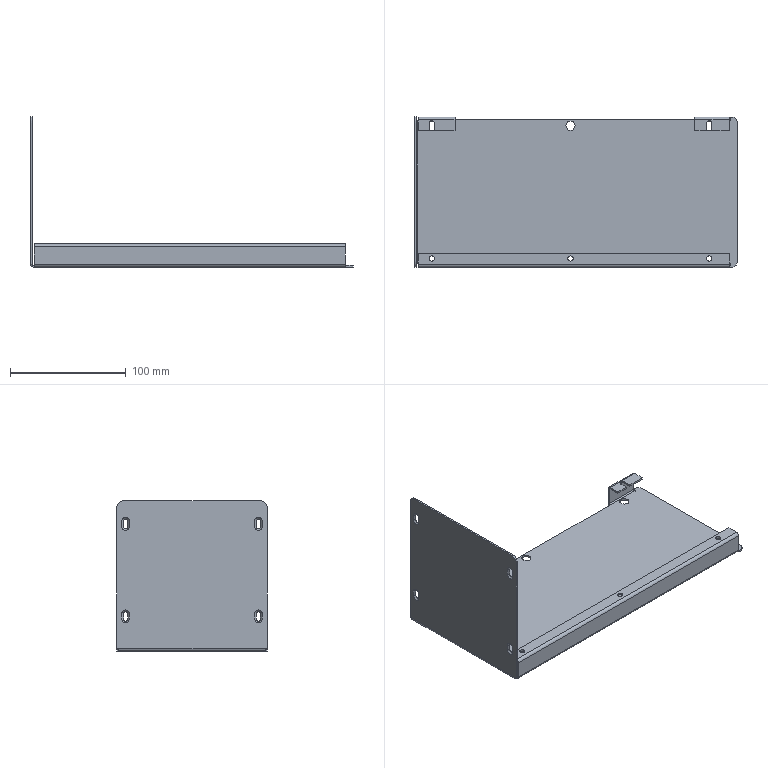Part | STEP file | FBDS-CS-004 | 1 solid | 126 faces | box 279.5 x 130 x 130 mm | volume 91348 mm3 | plane 74 | cylinder 38 | cone 12 | spline 2 | commonest cylinder face diameters 8 x12 4.5 x8 2 x7 5 x7 10 x4